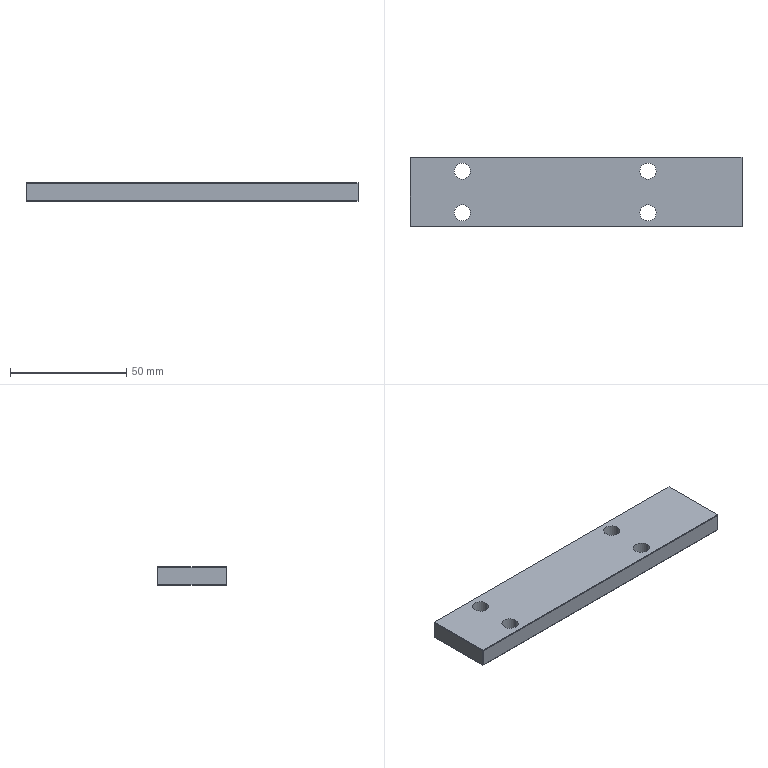Part | NX | 1 solid | 22 faces | box 143 x 30 x 8 mm | volume 33059 mm3 | plane 14 | cylinder 8 | commonest cylinder face diameters 7 x8
STEP:
#1=CARTESIAN_POINT('',(-62.2,14.7,-5.5));
#2=VERTEX_POINT('',#1);
#3=CARTESIAN_POINT('',(-62.2,-14.7,-5.5));
#4=VERTEX_POINT('',#3);
#5=CARTESIAN_POINT('',(-62.2,0.,-5.5));
#6=DIRECTION('',(0.,-1.,0.));
#7=VECTOR('',#6,1000.);
#8=LINE('',#5,#7);
#9=EDGE_CURVE('',#2,#4,#8,.T.);
#10=ORIENTED_EDGE('',*,*,#9,.F.);
#11=CARTESIAN_POINT('',(80.5,14.7,-5.5));
#12=VERTEX_POINT('',#11);
#13=CARTESIAN_POINT('',(0.,14.7,-5.5));
#14=DIRECTION('',(-1.,0.,0.));
#15=VECTOR('',#14,1000.);
#16=LINE('',#13,#15);
#17=EDGE_CURVE('',#12,#2,#16,.T.);
#18=ORIENTED_EDGE('',*,*,#17,.F.);
#19=CARTESIAN_POINT('',(80.5,-14.7,-5.5));
#20=VERTEX_POINT('',#19);
#21=CARTESIAN_POINT('',(80.5,0.,-5.5));
#22=DIRECTION('',(0.,1.,0.));
#23=VECTOR('',#22,1000.);
#24=LINE('',#21,#23);
#25=EDGE_CURVE('',#20,#12,#24,.T.);
#26=ORIENTED_EDGE('',*,*,#25,.F.);
#27=CARTESIAN_POINT('',(0.,-14.7,-5.5));
#28=DIRECTION('',(1.,0.,0.));
#29=VECTOR('',#28,1000.);
#30=LINE('',#27,#29);
#31=EDGE_CURVE('',#4,#20,#30,.T.);
#32=ORIENTED_EDGE('',*,*,#31,.F.);
#33=EDGE_LOOP('',(#10,#18,#26,#32));
#34=FACE_BOUND('',#33,.T.);
#35=CARTESIAN_POINT('',(36.5,9.,-5.5));
#36=VERTEX_POINT('',#35);
#37=CARTESIAN_POINT('',(43.5,9.,-5.5));
#38=VERTEX_POINT('',#37);
#39=CARTESIAN_POINT('',(40.,9.,-5.5));
#40=DIRECTION('',(0.,0.,1.));
#41=DIRECTION('',(1.,0.,0.));
#42=AXIS2_PLACEMENT_3D('',#39,#40,#41);
#43=CIRCLE('',#42,3.5);
#44=EDGE_CURVE('',#36,#38,#43,.T.);
#45=ORIENTED_EDGE('',*,*,#44,.T.);
#46=CARTESIAN_POINT('',(40.,9.,-5.5));
#47=DIRECTION('',(0.,0.,1.));
#48=DIRECTION('',(1.,0.,0.));
#49=AXIS2_PLACEMENT_3D('',#46,#47,#48);
#50=CIRCLE('',#49,3.5);
#51=EDGE_CURVE('',#38,#36,#50,.T.);
#52=ORIENTED_EDGE('',*,*,#51,.T.);
#53=EDGE_LOOP('',(#45,#52));
#54=FACE_BOUND('',#53,.T.);
#55=CARTESIAN_POINT('',(-43.5,9.,-5.5));
#56=VERTEX_POINT('',#55);
#57=CARTESIAN_POINT('',(-36.5,9.,-5.5));
#58=VERTEX_POINT('',#57);
#59=CARTESIAN_POINT('',(-40.,9.,-5.5));
#60=DIRECTION('',(0.,0.,1.));
#61=DIRECTION('',(1.,0.,0.));
#62=AXIS2_PLACEMENT_3D('',#59,#60,#61);
#63=CIRCLE('',#62,3.5);
#64=EDGE_CURVE('',#56,#58,#63,.T.);
#65=ORIENTED_EDGE('',*,*,#64,.T.);
#66=CARTESIAN_POINT('',(-40.,9.,-5.5));
#67=DIRECTION('',(0.,0.,1.));
#68=DIRECTION('',(1.,0.,0.));
#69=AXIS2_PLACEMENT_3D('',#66,#67,#68);
#70=CIRCLE('',#69,3.5);
#71=EDGE_CURVE('',#58,#56,#70,.T.);
#72=ORIENTED_EDGE('',*,*,#71,.T.);
#73=EDGE_LOOP('',(#65,#72));
#74=FACE_BOUND('',#73,.T.);
#75=CARTESIAN_POINT('',(36.5,-9.,-5.5));
#76=VERTEX_POINT('',#75);
#77=CARTESIAN_POINT('',(43.5,-9.,-5.5));
#78=VERTEX_POINT('',#77);
#79=CARTESIAN_POINT('',(40.,-9.,-5.5));
#80=DIRECTION('',(0.,0.,1.));
#81=DIRECTION('',(1.,0.,0.));
#82=AXIS2_PLACEMENT_3D('',#79,#80,#81);
#83=CIRCLE('',#82,3.5);
#84=EDGE_CURVE('',#76,#78,#83,.T.);
#85=ORIENTED_EDGE('',*,*,#84,.T.);
#86=CARTESIAN_POINT('',(40.,-9.,-5.5));
#87=DIRECTION('',(0.,0.,1.));
#88=DIRECTION('',(1.,0.,0.));
#89=AXIS2_PLACEMENT_3D('',#86,#87,#88);
#90=CIRCLE('',#89,3.5);
#91=EDGE_CURVE('',#78,#76,#90,.T.);
#92=ORIENTED_EDGE('',*,*,#91,.T.);
#93=EDGE_LOOP('',(#85,#92));
#94=FACE_BOUND('',#93,.T.);
#95=CARTESIAN_POINT('',(-43.5,-9.,-5.5));
#96=VERTEX_POINT('',#95);
#97=CARTESIAN_POINT('',(-36.5,-9.,-5.5));
#98=VERTEX_POINT('',#97);
#99=CARTESIAN_POINT('',(-40.,-9.,-5.5));
#100=DIRECTION('',(0.,0.,1.));
#101=DIRECTION('',(1.,0.,0.));
#102=AXIS2_PLACEMENT_3D('',#99,#100,#101);
#103=CIRCLE('',#102,3.5);
#104=EDGE_CURVE('',#96,#98,#103,.T.);
#105=ORIENTED_EDGE('',*,*,#104,.T.);
#106=CARTESIAN_POINT('',(-40.,-9.,-5.5));
#107=DIRECTION('',(0.,0.,1.));
#108=DIRECTION('',(1.,0.,0.));
#109=AXIS2_PLACEMENT_3D('',#106,#107,#108);
#110=CIRCLE('',#109,3.5);
#111=EDGE_CURVE('',#98,#96,#110,.T.);
#112=ORIENTED_EDGE('',*,*,#111,.T.);
#113=EDGE_LOOP('',(#105,#112));
#114=FACE_BOUND('',#113,.T.);
#115=CARTESIAN_POINT('',(0.,0.,-5.5));
#116=DIRECTION('',(0.,0.,1.));
#117=DIRECTION('',(1.,0.,0.));
#118=AXIS2_PLACEMENT_3D('',#115,#116,#117);
#119=PLANE('',#118);
#120=ADVANCED_FACE('',(#34,#54,#74,#94,#114),#119,.F.);
#121=CARTESIAN_POINT('',(-36.5,9.,2.5));
#122=VERTEX_POINT('',#121);
#123=CARTESIAN_POINT('',(-43.5,9.,2.5));
#124=VERTEX_POINT('',#123);
#125=CARTESIAN_POINT('',(-40.,9.,2.5));
#126=DIRECTION('',(0.,0.,1.));
#127=DIRECTION('',(-1.,0.,0.));
#128=AXIS2_PLACEMENT_3D('',#125,#126,#127);
#129=CIRCLE('',#128,3.5);
#130=EDGE_CURVE('',#122,#124,#129,.T.);
#131=ORIENTED_EDGE('',*,*,#130,.T.);
#132=CARTESIAN_POINT('',(-43.5,9.,-2.5));
#133=DIRECTION('',(0.,0.,1.));
#134=VECTOR('',#133,1000.);
#135=LINE('',#132,#134);
#136=EDGE_CURVE('',#124,#56,#135,.F.);
#137=ORIENTED_EDGE('',*,*,#136,.T.);
#138=ORIENTED_EDGE('',*,*,#71,.F.);
#139=CARTESIAN_POINT('',(-36.5,9.,-2.5));
#140=DIRECTION('',(0.,0.,1.));
#141=VECTOR('',#140,1000.);
#142=LINE('',#139,#141);
#143=EDGE_CURVE('',#122,#58,#142,.F.);
#144=ORIENTED_EDGE('',*,*,#143,.F.);
#145=EDGE_LOOP('',(#131,#137,#138,#144));
#146=FACE_BOUND('',#145,.T.);
#147=CARTESIAN_POINT('',(-40.,9.,-2.5));
#148=DIRECTION('',(0.,0.,1.));
#149=DIRECTION('',(1.,0.,0.));
#150=AXIS2_PLACEMENT_3D('',#147,#148,#149);
#151=CYLINDRICAL_SURFACE('',#150,3.5);
#152=ADVANCED_FACE('',(#146),#151,.F.);
#153=CARTESIAN_POINT('',(-62.5,-14.7,2.2));
#154=VERTEX_POINT('',#153);
#155=CARTESIAN_POINT('',(-62.5,-14.7,-5.2));
#156=VERTEX_POINT('',#155);
#157=CARTESIAN_POINT('',(-62.5,-14.7,-1.5));
#158=DIRECTION('',(0.,0.,-1.));
#159=VECTOR('',#158,1000.);
#160=LINE('',#157,#159);
#161=EDGE_CURVE('',#154,#156,#160,.T.);
#162=ORIENTED_EDGE('',*,*,#161,.F.);
#163=CARTESIAN_POINT('',(-62.5,14.7,2.2));
#164=VERTEX_POINT('',#163);
#165=CARTESIAN_POINT('',(-62.5,0.,2.2));
#166=DIRECTION('',(0.,-1.,0.));
#167=VECTOR('',#166,1000.);
#168=LINE('',#165,#167);
#169=EDGE_CURVE('',#164,#154,#168,.T.);
#170=ORIENTED_EDGE('',*,*,#169,.F.);
#171=CARTESIAN_POINT('',(-62.5,14.7,-5.2));
#172=VERTEX_POINT('',#171);
#173=CARTESIAN_POINT('',(-62.5,14.7,-1.5));
#174=DIRECTION('',(0.,0.,1.));
#175=VECTOR('',#174,1000.);
#176=LINE('',#173,#175);
#177=EDGE_CURVE('',#172,#164,#176,.T.);
#178=ORIENTED_EDGE('',*,*,#177,.F.);
#179=CARTESIAN_POINT('',(-62.5,0.,-5.2));
#180=DIRECTION('',(0.,-1.,0.));
#181=VECTOR('',#180,1000.);
#182=LINE('',#179,#181);
#183=EDGE_CURVE('',#172,#156,#182,.T.);
#184=ORIENTED_EDGE('',*,*,#183,.T.);
#185=EDGE_LOOP('',(#162,#170,#178,#184));
#186=FACE_BOUND('',#185,.T.);
#187=CARTESIAN_POINT('',(-62.5,15.,-2.5));
#188=DIRECTION('',(-1.,0.,0.));
#189=DIRECTION('',(0.,0.,1.));
#190=AXIS2_PLACEMENT_3D('',#187,#188,#189);
#191=PLANE('',#190);
#192=ADVANCED_FACE('',(#186),#191,.T.);
#193=CARTESIAN_POINT('',(-62.2,15.,2.2));
#194=VERTEX_POINT('',#193);
#195=CARTESIAN_POINT('',(80.5,15.,2.2));
#196=VERTEX_POINT('',#195);
#197=CARTESIAN_POINT('',(0.,15.,2.2));
#198=DIRECTION('',(1.,0.,0.));
#199=VECTOR('',#198,1000.);
#200=LINE('',#197,#199);
#201=EDGE_CURVE('',#194,#196,#200,.T.);
#202=ORIENTED_EDGE('',*,*,#201,.T.);
#203=CARTESIAN_POINT('',(80.5,15.,-5.2));
#204=VERTEX_POINT('',#203);
#205=CARTESIAN_POINT('',(80.5,15.,0.));
#206=DIRECTION('',(0.,0.,-1.));
#207=VECTOR('',#206,1000.);
#208=LINE('',#205,#207);
#209=EDGE_CURVE('',#196,#204,#208,.T.);
#210=ORIENTED_EDGE('',*,*,#209,.T.);
#211=CARTESIAN_POINT('',(-62.2,15.,-5.2));
#212=VERTEX_POINT('',#211);
#213=CARTESIAN_POINT('',(0.,15.,-5.2));
#214=DIRECTION('',(-1.,0.,0.));
#215=VECTOR('',#214,1000.);
#216=LINE('',#213,#215);
#217=EDGE_CURVE('',#204,#212,#216,.T.);
#218=ORIENTED_EDGE('',*,*,#217,.T.);
#219=CARTESIAN_POINT('',(-62.2,15.,-1.5));
#220=DIRECTION('',(0.,0.,1.));
#221=VECTOR('',#220,1000.);
#222=LINE('',#219,#221);
#223=EDGE_CURVE('',#212,#194,#222,.T.);
#224=ORIENTED_EDGE('',*,*,#223,.T.);
#225=EDGE_LOOP('',(#202,#210,#218,#224));
#226=FACE_BOUND('',#225,.T.);
#227=CARTESIAN_POINT('',(61.5,15.,-2.5));
#228=DIRECTION('',(0.,1.,0.));
#229=DIRECTION('',(1.,0.,0.));
#230=AXIS2_PLACEMENT_3D('',#227,#228,#229);
#231=PLANE('',#230);
#232=ADVANCED_FACE('',(#226),#231,.T.);
#233=ORIENTED_EDGE('',*,*,#25,.T.);
#234=CARTESIAN_POINT('',(80.5,0.,-20.2));
#235=DIRECTION('',(0.,0.7071,0.7071));
#236=VECTOR('',#235,1000.);
#237=LINE('',#234,#236);
#238=EDGE_CURVE('',#12,#204,#237,.T.);
#239=ORIENTED_EDGE('',*,*,#238,.T.);
#240=ORIENTED_EDGE('',*,*,#209,.F.);
#241=CARTESIAN_POINT('',(80.5,14.7,2.5));
#242=VERTEX_POINT('',#241);
#243=CARTESIAN_POINT('',(80.5,0.,17.2));
#244=DIRECTION('',(0.,0.7071,-0.7071));
#245=VECTOR('',#244,1000.);
#246=LINE('',#243,#245);
#247=EDGE_CURVE('',#242,#196,#246,.T.);
#248=ORIENTED_EDGE('',*,*,#247,.F.);
#249=CARTESIAN_POINT('',(80.5,-14.7,2.5));
#250=VERTEX_POINT('',#249);
#251=CARTESIAN_POINT('',(80.5,0.,2.5));
#252=DIRECTION('',(0.,1.,0.));
#253=VECTOR('',#252,1000.);
#254=LINE('',#251,#253);
#255=EDGE_CURVE('',#250,#242,#254,.T.);
#256=ORIENTED_EDGE('',*,*,#255,.F.);
#257=CARTESIAN_POINT('',(80.5,-15.,2.2));
#258=VERTEX_POINT('',#257);
#259=CARTESIAN_POINT('',(80.5,0.,17.2));
#260=DIRECTION('',(0.,0.7071,0.7071));
#261=VECTOR('',#260,1000.);
#262=LINE('',#259,#261);
#263=EDGE_CURVE('',#258,#250,#262,.T.);
#264=ORIENTED_EDGE('',*,*,#263,.F.);
#265=CARTESIAN_POINT('',(80.5,-15.,-5.2));
#266=VERTEX_POINT('',#265);
#267=CARTESIAN_POINT('',(80.5,-15.,0.));
#268=DIRECTION('',(0.,0.,1.));
#269=VECTOR('',#268,1000.);
#270=LINE('',#267,#269);
#271=EDGE_CURVE('',#266,#258,#270,.T.);
#272=ORIENTED_EDGE('',*,*,#271,.F.);
#273=CARTESIAN_POINT('',(80.5,0.,-20.2));
#274=DIRECTION('',(0.,0.7071,-0.7071));
#275=VECTOR('',#274,1000.);
#276=LINE('',#273,#275);
#277=EDGE_CURVE('',#266,#20,#276,.T.);
#278=ORIENTED_EDGE('',*,*,#277,.T.);
#279=EDGE_LOOP('',(#233,#239,#240,#248,#256,#264,#272,#278));
#280=FACE_BOUND('',#279,.T.);
#281=CARTESIAN_POINT('',(80.5,-15.,-2.5));
#282=DIRECTION('',(1.,0.,0.));
#283=DIRECTION('',(0.,1.,0.));
#284=AXIS2_PLACEMENT_3D('',#281,#282,#283);
#285=PLANE('',#284);
#286=ADVANCED_FACE('',(#280),#285,.T.);
#287=CARTESIAN_POINT('',(36.5,9.,2.5));
#288=VERTEX_POINT('',#287);
#289=CARTESIAN_POINT('',(43.5,9.,2.5));
#290=VERTEX_POINT('',#289);
#291=CARTESIAN_POINT('',(40.,9.,2.5));
#292=DIRECTION('',(0.,0.,1.));
#293=DIRECTION('',(-1.,0.,0.));
#294=AXIS2_PLACEMENT_3D('',#291,#292,#293);
#295=CIRCLE('',#294,3.5);
#296=EDGE_CURVE('',#288,#290,#295,.T.);
#297=ORIENTED_EDGE('',*,*,#296,.T.);
#298=CARTESIAN_POINT('',(43.5,9.,-2.5));
#299=DIRECTION('',(0.,0.,1.));
#300=VECTOR('',#299,1000.);
#301=LINE('',#298,#300);
#302=EDGE_CURVE('',#38,#290,#301,.T.);
#303=ORIENTED_EDGE('',*,*,#302,.F.);
#304=ORIENTED_EDGE('',*,*,#44,.F.);
#305=CARTESIAN_POINT('',(36.5,9.,-2.5));
#306=DIRECTION('',(0.,0.,1.));
#307=VECTOR('',#306,1000.);
#308=LINE('',#305,#307);
#309=EDGE_CURVE('',#36,#288,#308,.T.);
#310=ORIENTED_EDGE('',*,*,#309,.T.);
#311=EDGE_LOOP('',(#297,#303,#304,#310));
#312=FACE_BOUND('',#311,.T.);
#313=CARTESIAN_POINT('',(40.,9.,-2.5));
#314=DIRECTION('',(0.,0.,1.));
#315=DIRECTION('',(1.,0.,0.));
#316=AXIS2_PLACEMENT_3D('',#313,#314,#315);
#317=CYLINDRICAL_SURFACE('',#316,3.5);
#318=ADVANCED_FACE('',(#312),#317,.F.);
#319=CARTESIAN_POINT('',(36.5,-9.,2.5));
#320=VERTEX_POINT('',#319);
#321=CARTESIAN_POINT('',(43.5,-9.,2.5));
#322=VERTEX_POINT('',#321);
#323=CARTESIAN_POINT('',(40.,-9.,2.5));
#324=DIRECTION('',(0.,0.,1.));
#325=DIRECTION('',(-1.,0.,0.));
#326=AXIS2_PLACEMENT_3D('',#323,#324,#325);
#327=CIRCLE('',#326,3.5);
#328=EDGE_CURVE('',#320,#322,#327,.T.);
#329=ORIENTED_EDGE('',*,*,#328,.T.);
#330=CARTESIAN_POINT('',(43.5,-9.,-2.5));
#331=DIRECTION('',(0.,0.,1.));
#332=VECTOR('',#331,1000.);
#333=LINE('',#330,#332);
#334=EDGE_CURVE('',#78,#322,#333,.T.);
#335=ORIENTED_EDGE('',*,*,#334,.F.);
#336=ORIENTED_EDGE('',*,*,#84,.F.);
#337=CARTESIAN_POINT('',(36.5,-9.,-2.5));
#338=DIRECTION('',(0.,0.,1.));
#339=VECTOR('',#338,1000.);
#340=LINE('',#337,#339);
#341=EDGE_CURVE('',#76,#320,#340,.T.);
#342=ORIENTED_EDGE('',*,*,#341,.T.);
#343=EDGE_LOOP('',(#329,#335,#336,#342));
#344=FACE_BOUND('',#343,.T.);
#345=CARTESIAN_POINT('',(40.,-9.,-2.5));
#346=DIRECTION('',(0.,0.,1.));
#347=DIRECTION('',(1.,0.,0.));
#348=AXIS2_PLACEMENT_3D('',#345,#346,#347);
#349=CYLINDRICAL_SURFACE('',#348,3.5);
#350=ADVANCED_FACE('',(#344),#349,.F.);
#351=CARTESIAN_POINT('',(-36.5,-9.,2.5));
#352=VERTEX_POINT('',#351);
#353=CARTESIAN_POINT('',(-43.5,-9.,2.5));
#354=VERTEX_POINT('',#353);
#355=CARTESIAN_POINT('',(-40.,-9.,2.5));
#356=DIRECTION('',(0.,0.,1.));
#357=DIRECTION('',(-1.,0.,0.));
#358=AXIS2_PLACEMENT_3D('',#355,#356,#357);
#359=CIRCLE('',#358,3.5);
#360=EDGE_CURVE('',#352,#354,#359,.T.);
#361=ORIENTED_EDGE('',*,*,#360,.T.);
#362=CARTESIAN_POINT('',(-43.5,-9.,-2.5));
#363=DIRECTION('',(0.,0.,1.));
#364=VECTOR('',#363,1000.);
#365=LINE('',#362,#364);
#366=EDGE_CURVE('',#354,#96,#365,.F.);
#367=ORIENTED_EDGE('',*,*,#366,.T.);
#368=ORIENTED_EDGE('',*,*,#111,.F.);
#369=CARTESIAN_POINT('',(-36.5,-9.,-2.5));
#370=DIRECTION('',(0.,0.,1.));
#371=VECTOR('',#370,1000.);
#372=LINE('',#369,#371);
#373=EDGE_CURVE('',#352,#98,#372,.F.);
#374=ORIENTED_EDGE('',*,*,#373,.F.);
#375=EDGE_LOOP('',(#361,#367,#368,#374));
#376=FACE_BOUND('',#375,.T.);
#377=CARTESIAN_POINT('',(-40.,-9.,-2.5));
#378=DIRECTION('',(0.,0.,1.));
#379=DIRECTION('',(1.,0.,0.));
#380=AXIS2_PLACEMENT_3D('',#377,#378,#379);
#381=CYLINDRICAL_SURFACE('',#380,3.5);
#382=ADVANCED_FACE('',(#376),#381,.F.);
#383=CARTESIAN_POINT('',(-62.2,-15.,-5.2));
#384=VERTEX_POINT('',#383);
#385=CARTESIAN_POINT('',(0.,-15.,-5.2));
#386=DIRECTION('',(1.,0.,0.));
#387=VECTOR('',#386,1000.);
#388=LINE('',#385,#387);
#389=EDGE_CURVE('',#384,#266,#388,.T.);
#390=ORIENTED_EDGE('',*,*,#389,.T.);
#391=ORIENTED_EDGE('',*,*,#271,.T.);
#392=CARTESIAN_POINT('',(-62.2,-15.,2.2));
#393=VERTEX_POINT('',#392);
#394=CARTESIAN_POINT('',(0.,-15.,2.2));
#395=DIRECTION('',(-1.,0.,0.));
#396=VECTOR('',#395,1000.);
#397=LINE('',#394,#396);
#398=EDGE_CURVE('',#258,#393,#397,.T.);
#399=ORIENTED_EDGE('',*,*,#398,.T.);
#400=CARTESIAN_POINT('',(-62.2,-15.,-1.5));
#401=DIRECTION('',(0.,0.,-1.));
#402=VECTOR('',#401,1000.);
#403=LINE('',#400,#402);
#404=EDGE_CURVE('',#393,#384,#403,.T.);
#405=ORIENTED_EDGE('',*,*,#404,.T.);
#406=EDGE_LOOP('',(#390,#391,#399,#405));
#407=FACE_BOUND('',#406,.T.);
#408=CARTESIAN_POINT('',(-61.5,-15.,-2.5));
#409=DIRECTION('',(0.,-1.,0.));
#410=DIRECTION('',(0.,0.,-1.));
#411=AXIS2_PLACEMENT_3D('',#408,#409,#410);
#412=PLANE('',#411);
#413=ADVANCED_FACE('',(#407),#412,.T.);
#414=CARTESIAN_POINT('',(-62.2,-14.7,2.5));
#415=VERTEX_POINT('',#414);
#416=CARTESIAN_POINT('',(0.,-14.7,2.5));
#417=DIRECTION('',(-1.,0.,0.));
#418=VECTOR('',#417,1000.);
#419=LINE('',#416,#418);
#420=EDGE_CURVE('',#250,#415,#419,.T.);
#421=ORIENTED_EDGE('',*,*,#420,.F.);
#422=ORIENTED_EDGE('',*,*,#255,.T.);
#423=CARTESIAN_POINT('',(-62.2,14.7,2.5));
#424=VERTEX_POINT('',#423);
#425=CARTESIAN_POINT('',(0.,14.7,2.5));
#426=DIRECTION('',(1.,0.,0.));
#427=VECTOR('',#426,1000.);
#428=LINE('',#425,#427);
#429=EDGE_CURVE('',#424,#242,#428,.T.);
#430=ORIENTED_EDGE('',*,*,#429,.F.);
#431=CARTESIAN_POINT('',(-62.2,0.,2.5));
#432=DIRECTION('',(0.,-1.,0.));
#433=VECTOR('',#432,1000.);
#434=LINE('',#431,#433);
#435=EDGE_CURVE('',#424,#415,#434,.T.);
#436=ORIENTED_EDGE('',*,*,#435,.T.);
#437=EDGE_LOOP('',(#421,#422,#430,#436));
#438=FACE_BOUND('',#437,.T.);
#439=ORIENTED_EDGE('',*,*,#360,.F.);
#440=CARTESIAN_POINT('',(-40.,-9.,2.5));
#441=DIRECTION('',(0.,0.,1.));
#442=DIRECTION('',(-1.,0.,0.));
#443=AXIS2_PLACEMENT_3D('',#440,#441,#442);
#444=CIRCLE('',#443,3.5);
#445=EDGE_CURVE('',#354,#352,#444,.T.);
#446=ORIENTED_EDGE('',*,*,#445,.F.);
#447=EDGE_LOOP('',(#439,#446));
#448=FACE_BOUND('',#447,.T.);
#449=ORIENTED_EDGE('',*,*,#130,.F.);
#450=CARTESIAN_POINT('',(-40.,9.,2.5));
#451=DIRECTION('',(0.,0.,1.));
#452=DIRECTION('',(-1.,0.,0.));
#453=AXIS2_PLACEMENT_3D('',#450,#451,#452);
#454=CIRCLE('',#453,3.5);
#455=EDGE_CURVE('',#124,#122,#454,.T.);
#456=ORIENTED_EDGE('',*,*,#455,.F.);
#457=EDGE_LOOP('',(#449,#456));
#458=FACE_BOUND('',#457,.T.);
#459=ORIENTED_EDGE('',*,*,#328,.F.);
#460=CARTESIAN_POINT('',(40.,-9.,2.5));
#461=DIRECTION('',(0.,0.,1.));
#462=DIRECTION('',(-1.,0.,0.));
#463=AXIS2_PLACEMENT_3D('',#460,#461,#462);
#464=CIRCLE('',#463,3.5);
#465=EDGE_CURVE('',#322,#320,#464,.T.);
#466=ORIENTED_EDGE('',*,*,#465,.F.);
#467=EDGE_LOOP('',(#459,#466));
#468=FACE_BOUND('',#467,.T.);
#469=ORIENTED_EDGE('',*,*,#296,.F.);
#470=CARTESIAN_POINT('',(40.,9.,2.5));
#471=DIRECTION('',(0.,0.,1.));
#472=DIRECTION('',(-1.,0.,0.));
#473=AXIS2_PLACEMENT_3D('',#470,#471,#472);
#474=CIRCLE('',#473,3.5);
#475=EDGE_CURVE('',#290,#288,#474,.T.);
#476=ORIENTED_EDGE('',*,*,#475,.F.);
#477=EDGE_LOOP('',(#469,#476));
#478=FACE_BOUND('',#477,.T.);
#479=CARTESIAN_POINT('',(0.,0.,2.5));
#480=DIRECTION('',(0.,0.,1.));
#481=DIRECTION('',(1.,0.,0.));
#482=AXIS2_PLACEMENT_3D('',#479,#480,#481);
#483=PLANE('',#482);
#484=ADVANCED_FACE('',(#438,#448,#458,#468,#478),#483,.T.);
#485=ORIENTED_EDGE('',*,*,#201,.F.);
#486=CARTESIAN_POINT('',(-62.35,14.85,2.35));
#487=VERTEX_POINT('',#486);
#488=CARTESIAN_POINT('',(-77.2,0.,17.2));
#489=DIRECTION('',(-0.5774,-0.5774,0.5774));
#490=VECTOR('',#489,1000.);
#491=LINE('',#488,#490);
#492=EDGE_CURVE('',#194,#487,#491,.T.);
#493=ORIENTED_EDGE('',*,*,#492,.T.);
#494=CARTESIAN_POINT('',(-47.5,0.,17.2));
#495=DIRECTION('',(0.5774,-0.5774,0.5774));
#496=VECTOR('',#495,1000.);
#497=LINE('',#494,#496);
#498=EDGE_CURVE('',#487,#424,#497,.T.);
#499=ORIENTED_EDGE('',*,*,#498,.T.);
#500=ORIENTED_EDGE('',*,*,#429,.T.);
#501=ORIENTED_EDGE('',*,*,#247,.T.);
#502=EDGE_LOOP('',(#485,#493,#499,#500,#501));
#503=FACE_BOUND('',#502,.T.);
#504=CARTESIAN_POINT('',(0.15,14.85,2.35));
#505=DIRECTION('',(0.,0.7071,0.7071));
#506=DIRECTION('',(1.,0.,0.));
#507=AXIS2_PLACEMENT_3D('',#504,#505,#506);
#508=PLANE('',#507);
#509=ADVANCED_FACE('',(#503),#508,.T.);
#510=ORIENTED_EDGE('',*,*,#420,.T.);
#511=CARTESIAN_POINT('',(-62.35,-14.85,2.35));
#512=VERTEX_POINT('',#511);
#513=CARTESIAN_POINT('',(-47.5,0.,17.2));
#514=DIRECTION('',(-0.5774,-0.5774,-0.5774));
#515=VECTOR('',#514,1000.);
#516=LINE('',#513,#515);
#517=EDGE_CURVE('',#415,#512,#516,.T.);
#518=ORIENTED_EDGE('',*,*,#517,.T.);
#519=CARTESIAN_POINT('',(-77.2,0.,17.2));
#520=DIRECTION('',(0.5774,-0.5774,-0.5774));
#521=VECTOR('',#520,1000.);
#522=LINE('',#519,#521);
#523=EDGE_CURVE('',#512,#393,#522,.T.);
#524=ORIENTED_EDGE('',*,*,#523,.T.);
#525=ORIENTED_EDGE('',*,*,#398,.F.);
#526=ORIENTED_EDGE('',*,*,#263,.T.);
#527=EDGE_LOOP('',(#510,#518,#524,#525,#526));
#528=FACE_BOUND('',#527,.T.);
#529=CARTESIAN_POINT('',(0.15,-14.85,2.35));
#530=DIRECTION('',(0.,-0.7071,0.7071));
#531=DIRECTION('',(-1.,0.,0.));
#532=AXIS2_PLACEMENT_3D('',#529,#530,#531);
#533=PLANE('',#532);
#534=ADVANCED_FACE('',(#528),#533,.T.);
#535=ORIENTED_EDGE('',*,*,#17,.T.);
#536=CARTESIAN_POINT('',(-62.35,14.85,-5.35));
#537=VERTEX_POINT('',#536);
#538=CARTESIAN_POINT('',(-47.5,0.,-20.2));
#539=DIRECTION('',(-0.5774,0.5774,0.5774));
#540=VECTOR('',#539,1000.);
#541=LINE('',#538,#540);
#542=EDGE_CURVE('',#2,#537,#541,.T.);
#543=ORIENTED_EDGE('',*,*,#542,.T.);
#544=CARTESIAN_POINT('',(-77.2,0.,-20.2));
#545=DIRECTION('',(-0.5774,-0.5774,-0.5774));
#546=VECTOR('',#545,1000.);
#547=LINE('',#544,#546);
#548=EDGE_CURVE('',#212,#537,#547,.T.);
#549=ORIENTED_EDGE('',*,*,#548,.F.);
#550=ORIENTED_EDGE('',*,*,#217,.F.);
#551=ORIENTED_EDGE('',*,*,#238,.F.);
#552=EDGE_LOOP('',(#535,#543,#549,#550,#551));
#553=FACE_BOUND('',#552,.T.);
#554=CARTESIAN_POINT('',(0.15,14.85,-5.35));
#555=DIRECTION('',(0.,-0.7071,0.7071));
#556=DIRECTION('',(-1.,0.,0.));
#557=AXIS2_PLACEMENT_3D('',#554,#555,#556);
#558=PLANE('',#557);
#559=ADVANCED_FACE('',(#553),#558,.F.);
#560=ORIENTED_EDGE('',*,*,#389,.F.);
#561=CARTESIAN_POINT('',(-62.35,-14.85,-5.35));
#562=VERTEX_POINT('',#561);
#563=CARTESIAN_POINT('',(-77.2,0.,-20.2));
#564=DIRECTION('',(0.5774,-0.5774,0.5774));
#565=VECTOR('',#564,1000.);
#566=LINE('',#563,#565);
#567=EDGE_CURVE('',#562,#384,#566,.T.);
#568=ORIENTED_EDGE('',*,*,#567,.F.);
#569=CARTESIAN_POINT('',(-47.5,0.,-20.2));
#570=DIRECTION('',(0.5774,0.5774,-0.5774));
#571=VECTOR('',#570,1000.);
#572=LINE('',#569,#571);
#573=EDGE_CURVE('',#562,#4,#572,.T.);
#574=ORIENTED_EDGE('',*,*,#573,.T.);
#575=ORIENTED_EDGE('',*,*,#31,.T.);
#576=ORIENTED_EDGE('',*,*,#277,.F.);
#577=EDGE_LOOP('',(#560,#568,#574,#575,#576));
#578=FACE_BOUND('',#577,.T.);
#579=CARTESIAN_POINT('',(0.15,-14.85,-5.35));
#580=DIRECTION('',(0.,0.7071,0.7071));
#581=DIRECTION('',(1.,0.,0.));
#582=AXIS2_PLACEMENT_3D('',#579,#580,#581);
#583=PLANE('',#582);
#584=ADVANCED_FACE('',(#578),#583,.F.);
#585=ORIENTED_EDGE('',*,*,#183,.F.);
#586=CARTESIAN_POINT('',(-77.2,0.,9.5));
#587=DIRECTION('',(0.5774,0.5774,-0.5774));
#588=VECTOR('',#587,1000.);
#589=LINE('',#586,#588);
#590=EDGE_CURVE('',#172,#537,#589,.T.);
#591=ORIENTED_EDGE('',*,*,#590,.T.);
#592=ORIENTED_EDGE('',*,*,#542,.F.);
#593=ORIENTED_EDGE('',*,*,#9,.T.);
#594=ORIENTED_EDGE('',*,*,#573,.F.);
#595=CARTESIAN_POINT('',(-77.2,0.,9.5));
#596=DIRECTION('',(-0.5774,0.5774,0.5774));
#597=VECTOR('',#596,1000.);
#598=LINE('',#595,#597);
#599=EDGE_CURVE('',#562,#156,#598,.T.);
#600=ORIENTED_EDGE('',*,*,#599,.T.);
#601=EDGE_LOOP('',(#585,#591,#592,#593,#594,#600));
#602=FACE_BOUND('',#601,.T.);
#603=CARTESIAN_POINT('',(-62.35,0.,-5.35));
#604=DIRECTION('',(-0.7071,0.,-0.7071));
#605=DIRECTION('',(-0.7071,0.,0.7071));
#606=AXIS2_PLACEMENT_3D('',#603,#604,#605);
#607=PLANE('',#606);
#608=ADVANCED_FACE('',(#602),#607,.T.);
#609=ORIENTED_EDGE('',*,*,#177,.T.);
#610=CARTESIAN_POINT('',(-77.2,0.,-12.5));
#611=DIRECTION('',(-0.5774,-0.5774,-0.5774));
#612=VECTOR('',#611,1000.);
#613=LINE('',#610,#612);
#614=EDGE_CURVE('',#487,#164,#613,.T.);
#615=ORIENTED_EDGE('',*,*,#614,.F.);
#616=ORIENTED_EDGE('',*,*,#492,.F.);
#617=ORIENTED_EDGE('',*,*,#223,.F.);
#618=ORIENTED_EDGE('',*,*,#548,.T.);
#619=ORIENTED_EDGE('',*,*,#590,.F.);
#620=EDGE_LOOP('',(#609,#615,#616,#617,#618,#619));
#621=FACE_BOUND('',#620,.T.);
#622=CARTESIAN_POINT('',(-62.35,14.85,-1.5));
#623=DIRECTION('',(0.7071,-0.7071,0.));
#624=DIRECTION('',(0.,0.,-1.));
#625=AXIS2_PLACEMENT_3D('',#622,#623,#624);
#626=PLANE('',#625);
#627=ADVANCED_FACE('',(#621),#626,.F.);
#628=ORIENTED_EDGE('',*,*,#169,.T.);
#629=CARTESIAN_POINT('',(-77.2,0.,-12.5));
#630=DIRECTION('',(-0.5774,0.5774,-0.5774));
#631=VECTOR('',#630,1000.);
#632=LINE('',#629,#631);
#633=EDGE_CURVE('',#512,#154,#632,.T.);
#634=ORIENTED_EDGE('',*,*,#633,.F.);
#635=ORIENTED_EDGE('',*,*,#517,.F.);
#636=ORIENTED_EDGE('',*,*,#435,.F.);
#637=ORIENTED_EDGE('',*,*,#498,.F.);
#638=ORIENTED_EDGE('',*,*,#614,.T.);
#639=EDGE_LOOP('',(#628,#634,#635,#636,#637,#638));
#640=FACE_BOUND('',#639,.T.);
#641=CARTESIAN_POINT('',(-62.35,0.,2.35));
#642=DIRECTION('',(0.7071,0.,-0.7071));
#643=DIRECTION('',(0.,-1.,0.));
#644=AXIS2_PLACEMENT_3D('',#641,#642,#643);
#645=PLANE('',#644);
#646=ADVANCED_FACE('',(#640),#645,.F.);
#647=ORIENTED_EDGE('',*,*,#161,.T.);
#648=ORIENTED_EDGE('',*,*,#599,.F.);
#649=ORIENTED_EDGE('',*,*,#567,.T.);
#650=ORIENTED_EDGE('',*,*,#404,.F.);
#651=ORIENTED_EDGE('',*,*,#523,.F.);
#652=ORIENTED_EDGE('',*,*,#633,.T.);
#653=EDGE_LOOP('',(#647,#648,#649,#650,#651,#652));
#654=FACE_BOUND('',#653,.T.);
#655=CARTESIAN_POINT('',(-62.35,-14.85,-1.5));
#656=DIRECTION('',(0.7071,0.7071,0.));
#657=DIRECTION('',(0.,0.,-1.));
#658=AXIS2_PLACEMENT_3D('',#655,#656,#657);
#659=PLANE('',#658);
#660=ADVANCED_FACE('',(#654),#659,.F.);
#661=ORIENTED_EDGE('',*,*,#302,.T.);
#662=ORIENTED_EDGE('',*,*,#475,.T.);
#663=ORIENTED_EDGE('',*,*,#309,.F.);
#664=ORIENTED_EDGE('',*,*,#51,.F.);
#665=EDGE_LOOP('',(#661,#662,#663,#664));
#666=FACE_BOUND('',#665,.T.);
#667=CARTESIAN_POINT('',(40.,9.,-2.5));
#668=DIRECTION('',(0.,0.,1.));
#669=DIRECTION('',(1.,0.,0.));
#670=AXIS2_PLACEMENT_3D('',#667,#668,#669);
#671=CYLINDRICAL_SURFACE('',#670,3.5);
#672=ADVANCED_FACE('',(#666),#671,.F.);
#673=ORIENTED_EDGE('',*,*,#334,.T.);
#674=ORIENTED_EDGE('',*,*,#465,.T.);
#675=ORIENTED_EDGE('',*,*,#341,.F.);
#676=ORIENTED_EDGE('',*,*,#91,.F.);
#677=EDGE_LOOP('',(#673,#674,#675,#676));
#678=FACE_BOUND('',#677,.T.);
#679=CARTESIAN_POINT('',(40.,-9.,-2.5));
#680=DIRECTION('',(0.,0.,1.));
#681=DIRECTION('',(1.,0.,0.));
#682=AXIS2_PLACEMENT_3D('',#679,#680,#681);
#683=CYLINDRICAL_SURFACE('',#682,3.5);
#684=ADVANCED_FACE('',(#678),#683,.F.);
#685=ORIENTED_EDGE('',*,*,#104,.F.);
#686=ORIENTED_EDGE('',*,*,#366,.F.);
#687=ORIENTED_EDGE('',*,*,#445,.T.);
#688=ORIENTED_EDGE('',*,*,#373,.T.);
#689=EDGE_LOOP('',(#685,#686,#687,#688));
#690=FACE_BOUND('',#689,.T.);
#691=CARTESIAN_POINT('',(-40.,-9.,-2.5));
#692=DIRECTION('',(0.,0.,1.));
#693=DIRECTION('',(1.,0.,0.));
#694=AXIS2_PLACEMENT_3D('',#691,#692,#693);
#695=CYLINDRICAL_SURFACE('',#694,3.5);
#696=ADVANCED_FACE('',(#690),#695,.F.);
#697=ORIENTED_EDGE('',*,*,#64,.F.);
#698=ORIENTED_EDGE('',*,*,#136,.F.);
#699=ORIENTED_EDGE('',*,*,#455,.T.);
#700=ORIENTED_EDGE('',*,*,#143,.T.);
#701=EDGE_LOOP('',(#697,#698,#699,#700));
#702=FACE_BOUND('',#701,.T.);
#703=CARTESIAN_POINT('',(-40.,9.,-2.5));
#704=DIRECTION('',(0.,0.,1.));
#705=DIRECTION('',(1.,0.,0.));
#706=AXIS2_PLACEMENT_3D('',#703,#704,#705);
#707=CYLINDRICAL_SURFACE('',#706,3.5);
#708=ADVANCED_FACE('',(#702),#707,.F.);
#709=CLOSED_SHELL('',(#120,#152,#192,#232,#286,#318,#350,#382,#413,#484,#509,#534,#559,#584,#608,#627,#646,#660,#672,#684,#696,#708));
#710=MANIFOLD_SOLID_BREP('',#709);
#711=(LENGTH_UNIT()NAMED_UNIT(*)SI_UNIT(.MILLI.,.METRE.));
#712=UNCERTAINTY_MEASURE_WITH_UNIT(LENGTH_MEASURE(0.00001),#711,'','');
#713=(NAMED_UNIT(*)PLANE_ANGLE_UNIT()SI_UNIT($,.RADIAN.));
#714=(NAMED_UNIT(*)SI_UNIT($,.STERADIAN.)SOLID_ANGLE_UNIT());
#715=(GEOMETRIC_REPRESENTATION_CONTEXT(3)GLOBAL_UNCERTAINTY_ASSIGNED_CONTEXT((#712))GLOBAL_UNIT_ASSIGNED_CONTEXT((#711,#713,#714))REPRESENTATION_CONTEXT('',''));
#716=ADVANCED_BREP_SHAPE_REPRESENTATION('',(#710),#715);